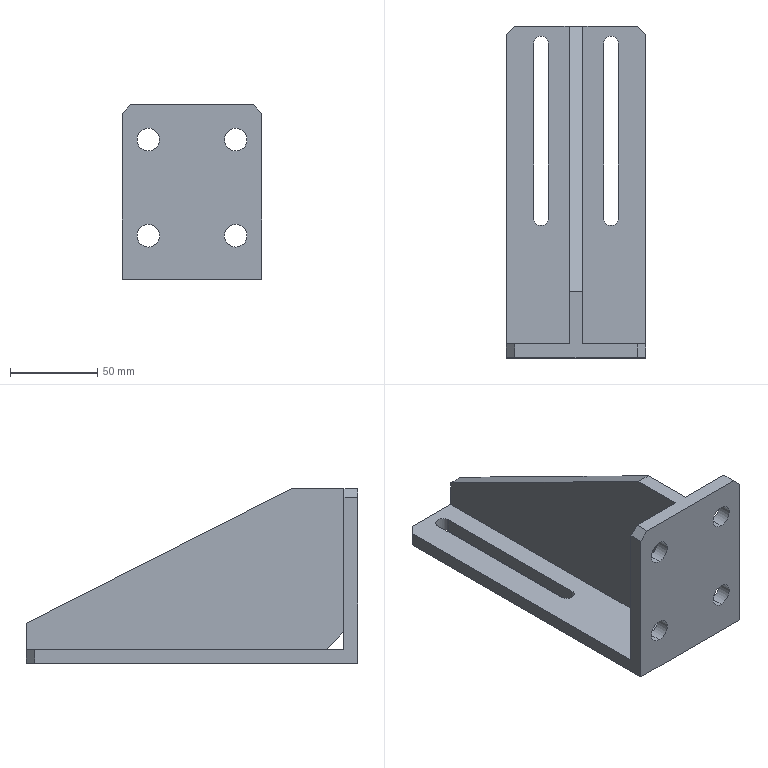Part | SolidWorks | features BaseBody 1 | 1 solid | 32 faces | box 80 x 190 x 100 mm | volume 248061 mm3 | plane 20 | cylinder 12 | commonest cylinder face diameters 13 x8 8.5 x4
STEP:
#1=CARTESIAN_POINT('',(-25.,-95.,18.5));
#2=VERTEX_POINT('',#1);
#3=CARTESIAN_POINT('',(-25.,-95.,31.5));
#4=VERTEX_POINT('',#3);
#5=CARTESIAN_POINT('',(-25.,-95.,25.));
#6=DIRECTION('',(0.,1.,0.));
#7=DIRECTION('',(0.,0.,1.));
#8=AXIS2_PLACEMENT_3D('',#5,#6,#7);
#9=CIRCLE('',#8,6.5);
#10=EDGE_CURVE('',#2,#4,#9,.T.);
#11=ORIENTED_EDGE('',*,*,#10,.F.);
#12=CARTESIAN_POINT('',(-25.,-87.,18.5));
#13=VERTEX_POINT('',#12);
#14=CARTESIAN_POINT('',(-25.,-87.,18.5));
#15=DIRECTION('',(0.,1.,0.));
#16=VECTOR('',#15,1000.);
#17=LINE('',#14,#16);
#18=EDGE_CURVE('',#2,#13,#17,.T.);
#19=ORIENTED_EDGE('',*,*,#18,.T.);
#20=CARTESIAN_POINT('',(-25.,-87.,31.5));
#21=VERTEX_POINT('',#20);
#22=CARTESIAN_POINT('',(-25.,-87.,25.));
#23=DIRECTION('',(0.,1.,0.));
#24=DIRECTION('',(0.,0.,1.));
#25=AXIS2_PLACEMENT_3D('',#22,#23,#24);
#26=CIRCLE('',#25,6.5);
#27=EDGE_CURVE('',#13,#21,#26,.T.);
#28=ORIENTED_EDGE('',*,*,#27,.T.);
#29=CARTESIAN_POINT('',(-25.,-87.,31.5));
#30=DIRECTION('',(0.,1.,0.));
#31=VECTOR('',#30,1000.);
#32=LINE('',#29,#31);
#33=EDGE_CURVE('',#4,#21,#32,.T.);
#34=ORIENTED_EDGE('',*,*,#33,.F.);
#35=EDGE_LOOP('',(#11,#19,#28,#34));
#36=FACE_OUTER_BOUND('',#35,.T.);
#37=CARTESIAN_POINT('',(-25.,-87.,25.));
#38=DIRECTION('',(0.,1.,0.));
#39=DIRECTION('',(0.,0.,1.));
#40=AXIS2_PLACEMENT_3D('',#37,#38,#39);
#41=CYLINDRICAL_SURFACE('',#40,6.5);
#42=ADVANCED_FACE('',(#36),#41,.F.);
#43=CARTESIAN_POINT('',(25.,-95.,18.5));
#44=VERTEX_POINT('',#43);
#45=CARTESIAN_POINT('',(25.,-95.,31.5));
#46=VERTEX_POINT('',#45);
#47=CARTESIAN_POINT('',(25.,-95.,25.));
#48=DIRECTION('',(0.,1.,0.));
#49=DIRECTION('',(0.,0.,1.));
#50=AXIS2_PLACEMENT_3D('',#47,#48,#49);
#51=CIRCLE('',#50,6.5);
#52=EDGE_CURVE('',#44,#46,#51,.T.);
#53=ORIENTED_EDGE('',*,*,#52,.F.);
#54=CARTESIAN_POINT('',(25.,-87.,18.5));
#55=VERTEX_POINT('',#54);
#56=CARTESIAN_POINT('',(25.,-87.,18.5));
#57=DIRECTION('',(0.,1.,0.));
#58=VECTOR('',#57,1000.);
#59=LINE('',#56,#58);
#60=EDGE_CURVE('',#44,#55,#59,.T.);
#61=ORIENTED_EDGE('',*,*,#60,.T.);
#62=CARTESIAN_POINT('',(25.,-87.,31.5));
#63=VERTEX_POINT('',#62);
#64=CARTESIAN_POINT('',(25.,-87.,25.));
#65=DIRECTION('',(0.,1.,0.));
#66=DIRECTION('',(0.,0.,1.));
#67=AXIS2_PLACEMENT_3D('',#64,#65,#66);
#68=CIRCLE('',#67,6.5);
#69=EDGE_CURVE('',#55,#63,#68,.T.);
#70=ORIENTED_EDGE('',*,*,#69,.T.);
#71=CARTESIAN_POINT('',(25.,-87.,31.5));
#72=DIRECTION('',(0.,1.,0.));
#73=VECTOR('',#72,1000.);
#74=LINE('',#71,#73);
#75=EDGE_CURVE('',#46,#63,#74,.T.);
#76=ORIENTED_EDGE('',*,*,#75,.F.);
#77=EDGE_LOOP('',(#53,#61,#70,#76));
#78=FACE_OUTER_BOUND('',#77,.T.);
#79=CARTESIAN_POINT('',(25.,-87.,25.));
#80=DIRECTION('',(0.,1.,0.));
#81=DIRECTION('',(0.,0.,1.));
#82=AXIS2_PLACEMENT_3D('',#79,#80,#81);
#83=CYLINDRICAL_SURFACE('',#82,6.5);
#84=ADVANCED_FACE('',(#78),#83,.F.);
#85=CARTESIAN_POINT('',(-25.,-95.,73.5));
#86=VERTEX_POINT('',#85);
#87=CARTESIAN_POINT('',(-25.,-95.,86.5));
#88=VERTEX_POINT('',#87);
#89=CARTESIAN_POINT('',(-25.,-95.,80.));
#90=DIRECTION('',(0.,1.,0.));
#91=DIRECTION('',(0.,0.,1.));
#92=AXIS2_PLACEMENT_3D('',#89,#90,#91);
#93=CIRCLE('',#92,6.5);
#94=EDGE_CURVE('',#86,#88,#93,.T.);
#95=ORIENTED_EDGE('',*,*,#94,.F.);
#96=CARTESIAN_POINT('',(-25.,-87.,73.5));
#97=VERTEX_POINT('',#96);
#98=CARTESIAN_POINT('',(-25.,-87.,73.5));
#99=DIRECTION('',(0.,1.,0.));
#100=VECTOR('',#99,1000.);
#101=LINE('',#98,#100);
#102=EDGE_CURVE('',#86,#97,#101,.T.);
#103=ORIENTED_EDGE('',*,*,#102,.T.);
#104=CARTESIAN_POINT('',(-25.,-87.,86.5));
#105=VERTEX_POINT('',#104);
#106=CARTESIAN_POINT('',(-25.,-87.,80.));
#107=DIRECTION('',(0.,1.,0.));
#108=DIRECTION('',(0.,0.,1.));
#109=AXIS2_PLACEMENT_3D('',#106,#107,#108);
#110=CIRCLE('',#109,6.5);
#111=EDGE_CURVE('',#97,#105,#110,.T.);
#112=ORIENTED_EDGE('',*,*,#111,.T.);
#113=CARTESIAN_POINT('',(-25.,-87.,86.5));
#114=DIRECTION('',(0.,1.,0.));
#115=VECTOR('',#114,1000.);
#116=LINE('',#113,#115);
#117=EDGE_CURVE('',#88,#105,#116,.T.);
#118=ORIENTED_EDGE('',*,*,#117,.F.);
#119=EDGE_LOOP('',(#95,#103,#112,#118));
#120=FACE_OUTER_BOUND('',#119,.T.);
#121=CARTESIAN_POINT('',(-25.,-87.,80.));
#122=DIRECTION('',(0.,1.,0.));
#123=DIRECTION('',(0.,0.,1.));
#124=AXIS2_PLACEMENT_3D('',#121,#122,#123);
#125=CYLINDRICAL_SURFACE('',#124,6.5);
#126=ADVANCED_FACE('',(#120),#125,.F.);
#127=CARTESIAN_POINT('',(25.,-95.,73.5));
#128=VERTEX_POINT('',#127);
#129=CARTESIAN_POINT('',(25.,-95.,86.5));
#130=VERTEX_POINT('',#129);
#131=CARTESIAN_POINT('',(25.,-95.,80.));
#132=DIRECTION('',(0.,1.,0.));
#133=DIRECTION('',(0.,0.,1.));
#134=AXIS2_PLACEMENT_3D('',#131,#132,#133);
#135=CIRCLE('',#134,6.5);
#136=EDGE_CURVE('',#128,#130,#135,.T.);
#137=ORIENTED_EDGE('',*,*,#136,.F.);
#138=CARTESIAN_POINT('',(25.,-87.,73.5));
#139=VERTEX_POINT('',#138);
#140=CARTESIAN_POINT('',(25.,-87.,73.5));
#141=DIRECTION('',(0.,1.,0.));
#142=VECTOR('',#141,1000.);
#143=LINE('',#140,#142);
#144=EDGE_CURVE('',#128,#139,#143,.T.);
#145=ORIENTED_EDGE('',*,*,#144,.T.);
#146=CARTESIAN_POINT('',(25.,-87.,86.5));
#147=VERTEX_POINT('',#146);
#148=CARTESIAN_POINT('',(25.,-87.,80.));
#149=DIRECTION('',(0.,1.,0.));
#150=DIRECTION('',(0.,0.,1.));
#151=AXIS2_PLACEMENT_3D('',#148,#149,#150);
#152=CIRCLE('',#151,6.5);
#153=EDGE_CURVE('',#139,#147,#152,.T.);
#154=ORIENTED_EDGE('',*,*,#153,.T.);
#155=CARTESIAN_POINT('',(25.,-87.,86.5));
#156=DIRECTION('',(0.,1.,0.));
#157=VECTOR('',#156,1000.);
#158=LINE('',#155,#157);
#159=EDGE_CURVE('',#130,#147,#158,.T.);
#160=ORIENTED_EDGE('',*,*,#159,.F.);
#161=EDGE_LOOP('',(#137,#145,#154,#160));
#162=FACE_OUTER_BOUND('',#161,.T.);
#163=CARTESIAN_POINT('',(25.,-87.,80.));
#164=DIRECTION('',(0.,1.,0.));
#165=DIRECTION('',(0.,0.,1.));
#166=AXIS2_PLACEMENT_3D('',#163,#164,#165);
#167=CYLINDRICAL_SURFACE('',#166,6.5);
#168=ADVANCED_FACE('',(#162),#167,.F.);
#169=CARTESIAN_POINT('',(-25.,-87.,25.));
#170=DIRECTION('',(0.,1.,0.));
#171=DIRECTION('',(0.,0.,1.));
#172=AXIS2_PLACEMENT_3D('',#169,#170,#171);
#173=CIRCLE('',#172,6.5);
#174=EDGE_CURVE('',#21,#13,#173,.T.);
#175=ORIENTED_EDGE('',*,*,#174,.F.);
#176=ORIENTED_EDGE('',*,*,#27,.F.);
#177=EDGE_LOOP('',(#175,#176));
#178=FACE_BOUND('',#177,.T.);
#179=CARTESIAN_POINT('',(25.,-87.,25.));
#180=DIRECTION('',(0.,1.,0.));
#181=DIRECTION('',(0.,0.,1.));
#182=AXIS2_PLACEMENT_3D('',#179,#180,#181);
#183=CIRCLE('',#182,6.5);
#184=EDGE_CURVE('',#63,#55,#183,.T.);
#185=ORIENTED_EDGE('',*,*,#184,.F.);
#186=ORIENTED_EDGE('',*,*,#69,.F.);
#187=EDGE_LOOP('',(#185,#186));
#188=FACE_BOUND('',#187,.T.);
#189=CARTESIAN_POINT('',(-40.,-87.,95.));
#190=VERTEX_POINT('',#189);
#191=CARTESIAN_POINT('',(-40.,-87.,8.));
#192=VERTEX_POINT('',#191);
#193=CARTESIAN_POINT('',(-40.,-87.,100.));
#194=DIRECTION('',(0.,0.,-1.));
#195=VECTOR('',#194,1000.);
#196=LINE('',#193,#195);
#197=EDGE_CURVE('',#190,#192,#196,.T.);
#198=ORIENTED_EDGE('',*,*,#197,.F.);
#199=CARTESIAN_POINT('',(-35.,-87.,100.));
#200=VERTEX_POINT('',#199);
#201=CARTESIAN_POINT('',(-35.,-87.,100.));
#202=DIRECTION('',(0.7071,0.,0.7071));
#203=VECTOR('',#202,1000.);
#204=LINE('',#201,#203);
#205=EDGE_CURVE('',#190,#200,#204,.T.);
#206=ORIENTED_EDGE('',*,*,#205,.T.);
#207=CARTESIAN_POINT('',(-4.,-87.,100.));
#208=VERTEX_POINT('',#207);
#209=CARTESIAN_POINT('',(-40.,-87.,100.));
#210=DIRECTION('',(-1.,0.,0.));
#211=VECTOR('',#210,1000.);
#212=LINE('',#209,#211);
#213=EDGE_CURVE('',#208,#200,#212,.T.);
#214=ORIENTED_EDGE('',*,*,#213,.F.);
#215=CARTESIAN_POINT('',(-4.,-87.,18.));
#216=VERTEX_POINT('',#215);
#217=CARTESIAN_POINT('',(-4.,-87.,18.));
#218=DIRECTION('',(0.,0.,1.));
#219=VECTOR('',#218,1000.);
#220=LINE('',#217,#219);
#221=EDGE_CURVE('',#216,#208,#220,.T.);
#222=ORIENTED_EDGE('',*,*,#221,.F.);
#223=CARTESIAN_POINT('',(4.,-87.,18.));
#224=VERTEX_POINT('',#223);
#225=CARTESIAN_POINT('',(-4.,-87.,18.));
#226=DIRECTION('',(1.,0.,0.));
#227=VECTOR('',#226,1000.);
#228=LINE('',#225,#227);
#229=EDGE_CURVE('',#216,#224,#228,.T.);
#230=ORIENTED_EDGE('',*,*,#229,.T.);
#231=CARTESIAN_POINT('',(4.,-87.,100.));
#232=VERTEX_POINT('',#231);
#233=CARTESIAN_POINT('',(4.,-87.,18.));
#234=DIRECTION('',(0.,0.,1.));
#235=VECTOR('',#234,1000.);
#236=LINE('',#233,#235);
#237=EDGE_CURVE('',#224,#232,#236,.T.);
#238=ORIENTED_EDGE('',*,*,#237,.T.);
#239=CARTESIAN_POINT('',(35.,-87.,100.));
#240=VERTEX_POINT('',#239);
#241=CARTESIAN_POINT('',(-40.,-87.,100.));
#242=DIRECTION('',(-1.,0.,0.));
#243=VECTOR('',#242,1000.);
#244=LINE('',#241,#243);
#245=EDGE_CURVE('',#240,#232,#244,.T.);
#246=ORIENTED_EDGE('',*,*,#245,.F.);
#247=CARTESIAN_POINT('',(40.,-87.,95.));
#248=VERTEX_POINT('',#247);
#249=CARTESIAN_POINT('',(35.,-87.,100.));
#250=DIRECTION('',(0.7071,0.,-0.7071));
#251=VECTOR('',#250,1000.);
#252=LINE('',#249,#251);
#253=EDGE_CURVE('',#240,#248,#252,.T.);
#254=ORIENTED_EDGE('',*,*,#253,.T.);
#255=CARTESIAN_POINT('',(40.,-87.,8.));
#256=VERTEX_POINT('',#255);
#257=CARTESIAN_POINT('',(40.,-87.,100.));
#258=DIRECTION('',(0.,0.,-1.));
#259=VECTOR('',#258,1000.);
#260=LINE('',#257,#259);
#261=EDGE_CURVE('',#248,#256,#260,.T.);
#262=ORIENTED_EDGE('',*,*,#261,.T.);
#263=CARTESIAN_POINT('',(-40.,-87.,8.));
#264=DIRECTION('',(-1.,0.,0.));
#265=VECTOR('',#264,1000.);
#266=LINE('',#263,#265);
#267=EDGE_CURVE('',#256,#192,#266,.T.);
#268=ORIENTED_EDGE('',*,*,#267,.T.);
#269=EDGE_LOOP('',(#198,#206,#214,#222,#230,#238,#246,#254,#262,#268));
#270=FACE_OUTER_BOUND('',#269,.T.);
#271=CARTESIAN_POINT('',(25.,-87.,80.));
#272=DIRECTION('',(0.,1.,0.));
#273=DIRECTION('',(0.,0.,1.));
#274=AXIS2_PLACEMENT_3D('',#271,#272,#273);
#275=CIRCLE('',#274,6.5);
#276=EDGE_CURVE('',#147,#139,#275,.T.);
#277=ORIENTED_EDGE('',*,*,#276,.F.);
#278=ORIENTED_EDGE('',*,*,#153,.F.);
#279=EDGE_LOOP('',(#277,#278));
#280=FACE_BOUND('',#279,.T.);
#281=CARTESIAN_POINT('',(-25.,-87.,80.));
#282=DIRECTION('',(0.,1.,0.));
#283=DIRECTION('',(0.,0.,1.));
#284=AXIS2_PLACEMENT_3D('',#281,#282,#283);
#285=CIRCLE('',#284,6.5);
#286=EDGE_CURVE('',#105,#97,#285,.T.);
#287=ORIENTED_EDGE('',*,*,#286,.F.);
#288=ORIENTED_EDGE('',*,*,#111,.F.);
#289=EDGE_LOOP('',(#287,#288));
#290=FACE_BOUND('',#289,.T.);
#291=CARTESIAN_POINT('',(-40.,-87.,100.));
#292=DIRECTION('',(0.,-1.,0.));
#293=DIRECTION('',(0.,0.,-1.));
#294=AXIS2_PLACEMENT_3D('',#291,#292,#293);
#295=PLANE('',#294);
#296=ADVANCED_FACE('',(#178,#188,#270,#280,#290),#295,.F.);
#297=CARTESIAN_POINT('',(15.75,85.,8.));
#298=VERTEX_POINT('',#297);
#299=CARTESIAN_POINT('',(15.75,-15.,8.));
#300=VERTEX_POINT('',#299);
#301=CARTESIAN_POINT('',(15.75,85.,8.));
#302=DIRECTION('',(0.,-1.,0.));
#303=VECTOR('',#302,1000.);
#304=LINE('',#301,#303);
#305=EDGE_CURVE('',#298,#300,#304,.T.);
#306=ORIENTED_EDGE('',*,*,#305,.F.);
#307=CARTESIAN_POINT('',(24.25,85.,8.));
#308=VERTEX_POINT('',#307);
#309=CARTESIAN_POINT('',(20.,85.,8.));
#310=DIRECTION('',(0.,0.,1.));
#311=DIRECTION('',(-1.,0.,0.));
#312=AXIS2_PLACEMENT_3D('',#309,#310,#311);
#313=CIRCLE('',#312,4.25);
#314=EDGE_CURVE('',#308,#298,#313,.T.);
#315=ORIENTED_EDGE('',*,*,#314,.F.);
#316=CARTESIAN_POINT('',(24.25,-15.,8.));
#317=VERTEX_POINT('',#316);
#318=CARTESIAN_POINT('',(24.25,85.,8.));
#319=DIRECTION('',(0.,1.,0.));
#320=VECTOR('',#319,1000.);
#321=LINE('',#318,#320);
#322=EDGE_CURVE('',#317,#308,#321,.T.);
#323=ORIENTED_EDGE('',*,*,#322,.F.);
#324=CARTESIAN_POINT('',(20.,-15.,8.));
#325=DIRECTION('',(0.,0.,1.));
#326=DIRECTION('',(-1.,0.,0.));
#327=AXIS2_PLACEMENT_3D('',#324,#325,#326);
#328=CIRCLE('',#327,4.25);
#329=EDGE_CURVE('',#300,#317,#328,.T.);
#330=ORIENTED_EDGE('',*,*,#329,.F.);
#331=EDGE_LOOP('',(#306,#315,#323,#330));
#332=FACE_BOUND('',#331,.T.);
#333=CARTESIAN_POINT('',(-24.25,85.,8.));
#334=VERTEX_POINT('',#333);
#335=CARTESIAN_POINT('',(-24.25,-15.,8.));
#336=VERTEX_POINT('',#335);
#337=CARTESIAN_POINT('',(-24.25,85.,8.));
#338=DIRECTION('',(0.,-1.,0.));
#339=VECTOR('',#338,1000.);
#340=LINE('',#337,#339);
#341=EDGE_CURVE('',#334,#336,#340,.T.);
#342=ORIENTED_EDGE('',*,*,#341,.F.);
#343=CARTESIAN_POINT('',(-15.75,85.,8.));
#344=VERTEX_POINT('',#343);
#345=CARTESIAN_POINT('',(-20.,85.,8.));
#346=DIRECTION('',(0.,0.,1.));
#347=DIRECTION('',(1.,0.,0.));
#348=AXIS2_PLACEMENT_3D('',#345,#346,#347);
#349=CIRCLE('',#348,4.25);
#350=EDGE_CURVE('',#344,#334,#349,.T.);
#351=ORIENTED_EDGE('',*,*,#350,.F.);
#352=CARTESIAN_POINT('',(-15.75,-15.,8.));
#353=VERTEX_POINT('',#352);
#354=CARTESIAN_POINT('',(-15.75,85.,8.));
#355=DIRECTION('',(0.,1.,0.));
#356=VECTOR('',#355,1000.);
#357=LINE('',#354,#356);
#358=EDGE_CURVE('',#353,#344,#357,.T.);
#359=ORIENTED_EDGE('',*,*,#358,.F.);
#360=CARTESIAN_POINT('',(-20.,-15.,8.));
#361=DIRECTION('',(0.,0.,1.));
#362=DIRECTION('',(1.,0.,0.));
#363=AXIS2_PLACEMENT_3D('',#360,#361,#362);
#364=CIRCLE('',#363,4.25);
#365=EDGE_CURVE('',#336,#353,#364,.T.);
#366=ORIENTED_EDGE('',*,*,#365,.F.);
#367=EDGE_LOOP('',(#342,#351,#359,#366));
#368=FACE_BOUND('',#367,.T.);
#369=CARTESIAN_POINT('',(40.,90.,8.));
#370=VERTEX_POINT('',#369);
#371=CARTESIAN_POINT('',(40.,95.,8.));
#372=DIRECTION('',(0.,1.,0.));
#373=VECTOR('',#372,1000.);
#374=LINE('',#371,#373);
#375=EDGE_CURVE('',#256,#370,#374,.T.);
#376=ORIENTED_EDGE('',*,*,#375,.T.);
#377=CARTESIAN_POINT('',(35.,95.,8.));
#378=VERTEX_POINT('',#377);
#379=CARTESIAN_POINT('',(35.,95.,8.));
#380=DIRECTION('',(-0.7071,0.7071,0.));
#381=VECTOR('',#380,1000.);
#382=LINE('',#379,#381);
#383=EDGE_CURVE('',#370,#378,#382,.T.);
#384=ORIENTED_EDGE('',*,*,#383,.T.);
#385=CARTESIAN_POINT('',(4.,95.,8.));
#386=VERTEX_POINT('',#385);
#387=CARTESIAN_POINT('',(40.,95.,8.));
#388=DIRECTION('',(-1.,0.,0.));
#389=VECTOR('',#388,1000.);
#390=LINE('',#387,#389);
#391=EDGE_CURVE('',#378,#386,#390,.T.);
#392=ORIENTED_EDGE('',*,*,#391,.T.);
#393=CARTESIAN_POINT('',(4.,-77.,8.));
#394=VERTEX_POINT('',#393);
#395=CARTESIAN_POINT('',(4.,95.,8.));
#396=DIRECTION('',(0.,-1.,0.));
#397=VECTOR('',#396,1000.);
#398=LINE('',#395,#397);
#399=EDGE_CURVE('',#386,#394,#398,.T.);
#400=ORIENTED_EDGE('',*,*,#399,.T.);
#401=CARTESIAN_POINT('',(-4.,-77.,8.));
#402=VERTEX_POINT('',#401);
#403=CARTESIAN_POINT('',(-4.,-77.,8.));
#404=DIRECTION('',(1.,0.,0.));
#405=VECTOR('',#404,1000.);
#406=LINE('',#403,#405);
#407=EDGE_CURVE('',#402,#394,#406,.T.);
#408=ORIENTED_EDGE('',*,*,#407,.F.);
#409=CARTESIAN_POINT('',(-4.,95.,8.));
#410=VERTEX_POINT('',#409);
#411=CARTESIAN_POINT('',(-4.,95.,8.));
#412=DIRECTION('',(0.,-1.,0.));
#413=VECTOR('',#412,1000.);
#414=LINE('',#411,#413);
#415=EDGE_CURVE('',#410,#402,#414,.T.);
#416=ORIENTED_EDGE('',*,*,#415,.F.);
#417=CARTESIAN_POINT('',(-35.,95.,8.));
#418=VERTEX_POINT('',#417);
#419=CARTESIAN_POINT('',(40.,95.,8.));
#420=DIRECTION('',(-1.,0.,0.));
#421=VECTOR('',#420,1000.);
#422=LINE('',#419,#421);
#423=EDGE_CURVE('',#410,#418,#422,.T.);
#424=ORIENTED_EDGE('',*,*,#423,.T.);
#425=CARTESIAN_POINT('',(-40.,90.,8.));
#426=VERTEX_POINT('',#425);
#427=CARTESIAN_POINT('',(-40.,90.,8.));
#428=DIRECTION('',(-0.7071,-0.7071,0.));
#429=VECTOR('',#428,1000.);
#430=LINE('',#427,#429);
#431=EDGE_CURVE('',#418,#426,#430,.T.);
#432=ORIENTED_EDGE('',*,*,#431,.T.);
#433=CARTESIAN_POINT('',(-40.,95.,8.));
#434=DIRECTION('',(0.,-1.,0.));
#435=VECTOR('',#434,1000.);
#436=LINE('',#433,#435);
#437=EDGE_CURVE('',#426,#192,#436,.T.);
#438=ORIENTED_EDGE('',*,*,#437,.T.);
#439=ORIENTED_EDGE('',*,*,#267,.F.);
#440=EDGE_LOOP('',(#376,#384,#392,#400,#408,#416,#424,#432,#438,#439));
#441=FACE_OUTER_BOUND('',#440,.T.);
#442=CARTESIAN_POINT('',(0.,0.,8.));
#443=DIRECTION('',(0.,0.,-1.));
#444=DIRECTION('',(-1.,0.,0.));
#445=AXIS2_PLACEMENT_3D('',#442,#443,#444);
#446=PLANE('',#445);
#447=ADVANCED_FACE('',(#332,#368,#441),#446,.F.);
#448=CARTESIAN_POINT('',(-40.,-95.,95.));
#449=VERTEX_POINT('',#448);
#450=CARTESIAN_POINT('',(-40.,-95.,0.));
#451=VERTEX_POINT('',#450);
#452=CARTESIAN_POINT('',(-40.,-95.,8.));
#453=DIRECTION('',(0.,0.,-1.));
#454=VECTOR('',#453,1000.);
#455=LINE('',#452,#454);
#456=EDGE_CURVE('',#449,#451,#455,.T.);
#457=ORIENTED_EDGE('',*,*,#456,.F.);
#458=CARTESIAN_POINT('',(-40.,95.,95.));
#459=DIRECTION('',(0.,1.,0.));
#460=VECTOR('',#459,1000.);
#461=LINE('',#458,#460);
#462=EDGE_CURVE('',#449,#190,#461,.T.);
#463=ORIENTED_EDGE('',*,*,#462,.T.);
#464=ORIENTED_EDGE('',*,*,#197,.T.);
#465=ORIENTED_EDGE('',*,*,#437,.F.);
#466=CARTESIAN_POINT('',(-40.,90.,0.));
#467=VERTEX_POINT('',#466);
#468=CARTESIAN_POINT('',(-40.,90.,8.));
#469=DIRECTION('',(0.,0.,-1.));
#470=VECTOR('',#469,1000.);
#471=LINE('',#468,#470);
#472=EDGE_CURVE('',#426,#467,#471,.T.);
#473=ORIENTED_EDGE('',*,*,#472,.T.);
#474=CARTESIAN_POINT('',(-40.,95.,0.));
#475=DIRECTION('',(0.,-1.,0.));
#476=VECTOR('',#475,1000.);
#477=LINE('',#474,#476);
#478=EDGE_CURVE('',#467,#451,#477,.T.);
#479=ORIENTED_EDGE('',*,*,#478,.T.);
#480=EDGE_LOOP('',(#457,#463,#464,#465,#473,#479));
#481=FACE_OUTER_BOUND('',#480,.T.);
#482=CARTESIAN_POINT('',(-40.,95.,8.));
#483=DIRECTION('',(1.,0.,0.));
#484=DIRECTION('',(0.,1.,0.));
#485=AXIS2_PLACEMENT_3D('',#482,#483,#484);
#486=PLANE('',#485);
#487=ADVANCED_FACE('',(#481),#486,.F.);
#488=CARTESIAN_POINT('',(-25.,-95.,25.));
#489=DIRECTION('',(0.,1.,0.));
#490=DIRECTION('',(0.,0.,1.));
#491=AXIS2_PLACEMENT_3D('',#488,#489,#490);
#492=CIRCLE('',#491,6.5);
#493=EDGE_CURVE('',#4,#2,#492,.T.);
#494=ORIENTED_EDGE('',*,*,#493,.T.);
#495=ORIENTED_EDGE('',*,*,#10,.T.);
#496=EDGE_LOOP('',(#494,#495));
#497=FACE_BOUND('',#496,.T.);
#498=CARTESIAN_POINT('',(25.,-95.,25.));
#499=DIRECTION('',(0.,1.,0.));
#500=DIRECTION('',(0.,0.,1.));
#501=AXIS2_PLACEMENT_3D('',#498,#499,#500);
#502=CIRCLE('',#501,6.5);
#503=EDGE_CURVE('',#46,#44,#502,.T.);
#504=ORIENTED_EDGE('',*,*,#503,.T.);
#505=ORIENTED_EDGE('',*,*,#52,.T.);
#506=EDGE_LOOP('',(#504,#505));
#507=FACE_BOUND('',#506,.T.);
#508=CARTESIAN_POINT('',(-25.,-95.,80.));
#509=DIRECTION('',(0.,1.,0.));
#510=DIRECTION('',(0.,0.,1.));
#511=AXIS2_PLACEMENT_3D('',#508,#509,#510);
#512=CIRCLE('',#511,6.5);
#513=EDGE_CURVE('',#88,#86,#512,.T.);
#514=ORIENTED_EDGE('',*,*,#513,.T.);
#515=ORIENTED_EDGE('',*,*,#94,.T.);
#516=EDGE_LOOP('',(#514,#515));
#517=FACE_BOUND('',#516,.T.);
#518=CARTESIAN_POINT('',(25.,-95.,80.));
#519=DIRECTION('',(0.,1.,0.));
#520=DIRECTION('',(0.,0.,1.));
#521=AXIS2_PLACEMENT_3D('',#518,#519,#520);
#522=CIRCLE('',#521,6.5);
#523=EDGE_CURVE('',#130,#128,#522,.T.);
#524=ORIENTED_EDGE('',*,*,#523,.T.);
#525=ORIENTED_EDGE('',*,*,#136,.T.);
#526=EDGE_LOOP('',(#524,#525));
#527=FACE_BOUND('',#526,.T.);
#528=CARTESIAN_POINT('',(-35.,-95.,100.));
#529=VERTEX_POINT('',#528);
#530=CARTESIAN_POINT('',(35.,-95.,100.));
#531=VERTEX_POINT('',#530);
#532=CARTESIAN_POINT('',(-40.,-95.,100.));
#533=DIRECTION('',(1.,0.,0.));
#534=VECTOR('',#533,1000.);
#535=LINE('',#532,#534);
#536=EDGE_CURVE('',#529,#531,#535,.T.);
#537=ORIENTED_EDGE('',*,*,#536,.F.);
#538=CARTESIAN_POINT('',(-35.,-95.,100.));
#539=DIRECTION('',(-0.7071,0.,-0.7071));
#540=VECTOR('',#539,1000.);
#541=LINE('',#538,#540);
#542=EDGE_CURVE('',#529,#449,#541,.T.);
#543=ORIENTED_EDGE('',*,*,#542,.T.);
#544=ORIENTED_EDGE('',*,*,#456,.T.);
#545=CARTESIAN_POINT('',(40.,-95.,0.));
#546=VERTEX_POINT('',#545);
#547=CARTESIAN_POINT('',(40.,-95.,0.));
#548=DIRECTION('',(1.,0.,0.));
#549=VECTOR('',#548,1000.);
#550=LINE('',#547,#549);
#551=EDGE_CURVE('',#451,#546,#550,.T.);
#552=ORIENTED_EDGE('',*,*,#551,.T.);
#553=CARTESIAN_POINT('',(40.,-95.,95.));
#554=VERTEX_POINT('',#553);
#555=CARTESIAN_POINT('',(40.,-95.,8.));
#556=DIRECTION('',(0.,0.,-1.));
#557=VECTOR('',#556,1000.);
#558=LINE('',#555,#557);
#559=EDGE_CURVE('',#554,#546,#558,.T.);
#560=ORIENTED_EDGE('',*,*,#559,.F.);
#561=CARTESIAN_POINT('',(35.,-95.,100.));
#562=DIRECTION('',(-0.7071,0.,0.7071));
#563=VECTOR('',#562,1000.);
#564=LINE('',#561,#563);
#565=EDGE_CURVE('',#554,#531,#564,.T.);
#566=ORIENTED_EDGE('',*,*,#565,.T.);
#567=EDGE_LOOP('',(#537,#543,#544,#552,#560,#566));
#568=FACE_OUTER_BOUND('',#567,.T.);
#569=CARTESIAN_POINT('',(40.,-95.,8.));
#570=DIRECTION('',(0.,1.,0.));
#571=DIRECTION('',(0.,0.,1.));
#572=AXIS2_PLACEMENT_3D('',#569,#570,#571);
#573=PLANE('',#572);
#574=ADVANCED_FACE('',(#497,#507,#517,#527,#568),#573,.F.);
#575=ORIENTED_EDGE('',*,*,#261,.F.);
#576=CARTESIAN_POINT('',(40.,95.,95.));
#577=DIRECTION('',(0.,-1.,0.));
#578=VECTOR('',#577,1000.);
#579=LINE('',#576,#578);
#580=EDGE_CURVE('',#248,#554,#579,.T.);
#581=ORIENTED_EDGE('',*,*,#580,.T.);
#582=ORIENTED_EDGE('',*,*,#559,.T.);
#583=CARTESIAN_POINT('',(40.,90.,0.));
#584=VERTEX_POINT('',#583);
#585=CARTESIAN_POINT('',(40.,95.,0.));
#586=DIRECTION('',(0.,1.,0.));
#587=VECTOR('',#586,1000.);
#588=LINE('',#585,#587);
#589=EDGE_CURVE('',#546,#584,#588,.T.);
#590=ORIENTED_EDGE('',*,*,#589,.T.);
#591=CARTESIAN_POINT('',(40.,90.,8.));
#592=DIRECTION('',(0.,0.,1.));
#593=VECTOR('',#592,1000.);
#594=LINE('',#591,#593);
#595=EDGE_CURVE('',#584,#370,#594,.T.);
#596=ORIENTED_EDGE('',*,*,#595,.T.);
#597=ORIENTED_EDGE('',*,*,#375,.F.);
#598=EDGE_LOOP('',(#575,#581,#582,#590,#596,#597));
#599=FACE_OUTER_BOUND('',#598,.T.);
#600=CARTESIAN_POINT('',(40.,95.,8.));
#601=DIRECTION('',(-1.,0.,0.));
#602=DIRECTION('',(0.,-1.,0.));
#603=AXIS2_PLACEMENT_3D('',#600,#601,#602);
#604=PLANE('',#603);
#605=ADVANCED_FACE('',(#599),#604,.F.);
#606=ORIENTED_EDGE('',*,*,#391,.F.);
#607=CARTESIAN_POINT('',(35.,95.,0.));
#608=VERTEX_POINT('',#607);
#609=CARTESIAN_POINT('',(35.,95.,8.));
#610=DIRECTION('',(0.,0.,-1.));
#611=VECTOR('',#610,1000.);
#612=LINE('',#609,#611);
#613=EDGE_CURVE('',#378,#608,#612,.T.);
#614=ORIENTED_EDGE('',*,*,#613,.T.);
#615=CARTESIAN_POINT('',(-35.,95.,0.));
#616=VERTEX_POINT('',#615);
#617=CARTESIAN_POINT('',(40.,95.,0.));
#618=DIRECTION('',(-1.,0.,0.));
#619=VECTOR('',#618,1000.);
#620=LINE('',#617,#619);
#621=EDGE_CURVE('',#608,#616,#620,.T.);
#622=ORIENTED_EDGE('',*,*,#621,.T.);
#623=CARTESIAN_POINT('',(-35.,95.,8.));
#624=DIRECTION('',(0.,0.,1.));
#625=VECTOR('',#624,1000.);
#626=LINE('',#623,#625);
#627=EDGE_CURVE('',#616,#418,#626,.T.);
#628=ORIENTED_EDGE('',*,*,#627,.T.);
#629=ORIENTED_EDGE('',*,*,#423,.F.);
#630=CARTESIAN_POINT('',(-4.,95.,23.));
#631=VERTEX_POINT('',#630);
#632=CARTESIAN_POINT('',(-4.,95.,8.));
#633=DIRECTION('',(0.,0.,-1.));
#634=VECTOR('',#633,1000.);
#635=LINE('',#632,#634);
#636=EDGE_CURVE('',#631,#410,#635,.T.);
#637=ORIENTED_EDGE('',*,*,#636,.F.);
#638=CARTESIAN_POINT('',(4.,95.,23.));
#639=VERTEX_POINT('',#638);
#640=CARTESIAN_POINT('',(-4.,95.,23.));
#641=DIRECTION('',(1.,0.,0.));
#642=VECTOR('',#641,1000.);
#643=LINE('',#640,#642);
#644=EDGE_CURVE('',#631,#639,#643,.T.);
#645=ORIENTED_EDGE('',*,*,#644,.T.);
#646=CARTESIAN_POINT('',(4.,95.,8.));
#647=DIRECTION('',(0.,0.,-1.));
#648=VECTOR('',#647,1000.);
#649=LINE('',#646,#648);
#650=EDGE_CURVE('',#639,#386,#649,.T.);
#651=ORIENTED_EDGE('',*,*,#650,.T.);
#652=EDGE_LOOP('',(#606,#614,#622,#628,#629,#637,#645,#651));
#653=FACE_OUTER_BOUND('',#652,.T.);
#654=CARTESIAN_POINT('',(40.,95.,8.));
#655=DIRECTION('',(0.,-1.,0.));
#656=DIRECTION('',(0.,0.,-1.));
#657=AXIS2_PLACEMENT_3D('',#654,#655,#656);
#658=PLANE('',#657);
#659=ADVANCED_FACE('',(#653),#658,.F.);
#660=CARTESIAN_POINT('',(24.25,85.,0.));
#661=VERTEX_POINT('',#660);
#662=CARTESIAN_POINT('',(15.75,85.,0.));
#663=VERTEX_POINT('',#662);
#664=CARTESIAN_POINT('',(20.,85.,0.));
#665=DIRECTION('',(0.,0.,1.));
#666=DIRECTION('',(-1.,0.,0.));
#667=AXIS2_PLACEMENT_3D('',#664,#665,#666);
#668=CIRCLE('',#667,4.25);
#669=EDGE_CURVE('',#661,#663,#668,.T.);
#670=ORIENTED_EDGE('',*,*,#669,.T.);
#671=CARTESIAN_POINT('',(15.75,-15.,0.));
#672=VERTEX_POINT('',#671);
#673=CARTESIAN_POINT('',(15.75,85.,0.));
#674=DIRECTION('',(0.,-1.,0.));
#675=VECTOR('',#674,1000.);
#676=LINE('',#673,#675);
#677=EDGE_CURVE('',#663,#672,#676,.T.);
#678=ORIENTED_EDGE('',*,*,#677,.T.);
#679=CARTESIAN_POINT('',(24.25,-15.,0.));
#680=VERTEX_POINT('',#679);
#681=CARTESIAN_POINT('',(20.,-15.,0.));
#682=DIRECTION('',(0.,0.,1.));
#683=DIRECTION('',(-1.,0.,0.));
#684=AXIS2_PLACEMENT_3D('',#681,#682,#683);
#685=CIRCLE('',#684,4.25);
#686=EDGE_CURVE('',#672,#680,#685,.T.);
#687=ORIENTED_EDGE('',*,*,#686,.T.);
#688=CARTESIAN_POINT('',(24.25,85.,0.));
#689=DIRECTION('',(0.,1.,0.));
#690=VECTOR('',#689,1000.);
#691=LINE('',#688,#690);
#692=EDGE_CURVE('',#680,#661,#691,.T.);
#693=ORIENTED_EDGE('',*,*,#692,.T.);
#694=EDGE_LOOP('',(#670,#678,#687,#693));
#695=FACE_BOUND('',#694,.T.);
#696=CARTESIAN_POINT('',(-15.75,85.,0.));
#697=VERTEX_POINT('',#696);
#698=CARTESIAN_POINT('',(-24.25,85.,0.));
#699=VERTEX_POINT('',#698);
#700=CARTESIAN_POINT('',(-20.,85.,0.));
#701=DIRECTION('',(0.,0.,1.));
#702=DIRECTION('',(1.,0.,0.));
#703=AXIS2_PLACEMENT_3D('',#700,#701,#702);
#704=CIRCLE('',#703,4.25);
#705=EDGE_CURVE('',#697,#699,#704,.T.);
#706=ORIENTED_EDGE('',*,*,#705,.T.);
#707=CARTESIAN_POINT('',(-24.25,-15.,0.));
#708=VERTEX_POINT('',#707);
#709=CARTESIAN_POINT('',(-24.25,85.,0.));
#710=DIRECTION('',(0.,-1.,0.));
#711=VECTOR('',#710,1000.);
#712=LINE('',#709,#711);
#713=EDGE_CURVE('',#699,#708,#712,.T.);
#714=ORIENTED_EDGE('',*,*,#713,.T.);
#715=CARTESIAN_POINT('',(-15.75,-15.,0.));
#716=VERTEX_POINT('',#715);
#717=CARTESIAN_POINT('',(-20.,-15.,0.));
#718=DIRECTION('',(0.,0.,1.));
#719=DIRECTION('',(1.,0.,0.));
#720=AXIS2_PLACEMENT_3D('',#717,#718,#719);
#721=CIRCLE('',#720,4.25);
#722=EDGE_CURVE('',#708,#716,#721,.T.);
#723=ORIENTED_EDGE('',*,*,#722,.T.);
#724=CARTESIAN_POINT('',(-15.75,85.,0.));
#725=DIRECTION('',(0.,1.,0.));
#726=VECTOR('',#725,1000.);
#727=LINE('',#724,#726);
#728=EDGE_CURVE('',#716,#697,#727,.T.);
#729=ORIENTED_EDGE('',*,*,#728,.T.);
#730=EDGE_LOOP('',(#706,#714,#723,#729));
#731=FACE_BOUND('',#730,.T.);
#732=ORIENTED_EDGE('',*,*,#621,.F.);
#733=CARTESIAN_POINT('',(65.,65.,0.));
#734=DIRECTION('',(0.7071,-0.7071,0.));
#735=VECTOR('',#734,1000.);
#736=LINE('',#733,#735);
#737=EDGE_CURVE('',#608,#584,#736,.T.);
#738=ORIENTED_EDGE('',*,*,#737,.T.);
#739=ORIENTED_EDGE('',*,*,#589,.F.);
#740=ORIENTED_EDGE('',*,*,#551,.F.);
#741=ORIENTED_EDGE('',*,*,#478,.F.);
#742=CARTESIAN_POINT('',(-65.,65.,0.));
#743=DIRECTION('',(0.7071,0.7071,0.));
#744=VECTOR('',#743,1000.);
#745=LINE('',#742,#744);
#746=EDGE_CURVE('',#467,#616,#745,.T.);
#747=ORIENTED_EDGE('',*,*,#746,.T.);
#748=EDGE_LOOP('',(#732,#738,#739,#740,#741,#747));
#749=FACE_OUTER_BOUND('',#748,.T.);
#750=CARTESIAN_POINT('',(0.,0.,0.));
#751=DIRECTION('',(0.,0.,-1.));
#752=DIRECTION('',(-1.,0.,0.));
#753=AXIS2_PLACEMENT_3D('',#750,#751,#752);
#754=PLANE('',#753);
#755=ADVANCED_FACE('',(#695,#731,#749),#754,.T.);
#756=ORIENTED_EDGE('',*,*,#213,.T.);
#757=CARTESIAN_POINT('',(-35.,0.,100.));
#758=DIRECTION('',(0.,-1.,0.));
#759=VECTOR('',#758,1000.);
#760=LINE('',#757,#759);
#761=EDGE_CURVE('',#200,#529,#760,.T.);
#762=ORIENTED_EDGE('',*,*,#761,.T.);
#763=ORIENTED_EDGE('',*,*,#536,.T.);
#764=CARTESIAN_POINT('',(35.,0.,100.));
#765=DIRECTION('',(0.,1.,0.));
#766=VECTOR('',#765,1000.);
#767=LINE('',#764,#766);
#768=EDGE_CURVE('',#531,#240,#767,.T.);
#769=ORIENTED_EDGE('',*,*,#768,.T.);
#770=ORIENTED_EDGE('',*,*,#245,.T.);
#771=CARTESIAN_POINT('',(4.,-57.,100.));
#772=VERTEX_POINT('',#771);
#773=CARTESIAN_POINT('',(4.,-57.,100.));
#774=DIRECTION('',(0.,1.,0.));
#775=VECTOR('',#774,1000.);
#776=LINE('',#773,#775);
#777=EDGE_CURVE('',#232,#772,#776,.T.);
#778=ORIENTED_EDGE('',*,*,#777,.T.);
#779=CARTESIAN_POINT('',(-4.,-57.,100.));
#780=VERTEX_POINT('',#779);
#781=CARTESIAN_POINT('',(-4.,-57.,100.));
#782=DIRECTION('',(1.,0.,0.));
#783=VECTOR('',#782,1000.);
#784=LINE('',#781,#783);
#785=EDGE_CURVE('',#780,#772,#784,.T.);
#786=ORIENTED_EDGE('',*,*,#785,.F.);
#787=CARTESIAN_POINT('',(-4.,-57.,100.));
#788=DIRECTION('',(0.,1.,0.));
#789=VECTOR('',#788,1000.);
#790=LINE('',#787,#789);
#791=EDGE_CURVE('',#208,#780,#790,.T.);
#792=ORIENTED_EDGE('',*,*,#791,.F.);
#793=EDGE_LOOP('',(#756,#762,#763,#769,#770,#778,#786,#792));
#794=FACE_OUTER_BOUND('',#793,.T.);
#795=CARTESIAN_POINT('',(0.,0.,100.));
#796=DIRECTION('',(0.,0.,-1.));
#797=DIRECTION('',(-1.,0.,0.));
#798=AXIS2_PLACEMENT_3D('',#795,#796,#797);
#799=PLANE('',#798);
#800=ADVANCED_FACE('',(#794),#799,.F.);
#801=CARTESIAN_POINT('',(4.,-77.,8.));
#802=DIRECTION('',(0.,-0.7071,0.7071));
#803=VECTOR('',#802,1000.);
#804=LINE('',#801,#803);
#805=EDGE_CURVE('',#394,#224,#804,.T.);
#806=ORIENTED_EDGE('',*,*,#805,.T.);
#807=ORIENTED_EDGE('',*,*,#229,.F.);
#808=CARTESIAN_POINT('',(-4.,-77.,8.));
#809=DIRECTION('',(0.,-0.7071,0.7071));
#810=VECTOR('',#809,1000.);
#811=LINE('',#808,#810);
#812=EDGE_CURVE('',#402,#216,#811,.T.);
#813=ORIENTED_EDGE('',*,*,#812,.F.);
#814=ORIENTED_EDGE('',*,*,#407,.T.);
#815=EDGE_LOOP('',(#806,#807,#813,#814));
#816=FACE_OUTER_BOUND('',#815,.T.);
#817=CARTESIAN_POINT('',(-4.,-77.,8.));
#818=DIRECTION('',(0.,0.7071,0.7071));
#819=DIRECTION('',(0.,-0.7071,0.7071));
#820=AXIS2_PLACEMENT_3D('',#817,#818,#819);
#821=PLANE('',#820);
#822=ADVANCED_FACE('',(#816),#821,.F.);
#823=CARTESIAN_POINT('',(4.,95.,23.));
#824=DIRECTION('',(0.,0.8921,-0.4519));
#825=VECTOR('',#824,1000.);
#826=LINE('',#823,#825);
#827=EDGE_CURVE('',#772,#639,#826,.T.);
#828=ORIENTED_EDGE('',*,*,#827,.T.);
#829=ORIENTED_EDGE('',*,*,#644,.F.);
#830=CARTESIAN_POINT('',(-4.,95.,23.));
#831=DIRECTION('',(0.,0.8921,-0.4519));
#832=VECTOR('',#831,1000.);
#833=LINE('',#830,#832);
#834=EDGE_CURVE('',#780,#631,#833,.T.);
#835=ORIENTED_EDGE('',*,*,#834,.F.);
#836=ORIENTED_EDGE('',*,*,#785,.T.);
#837=EDGE_LOOP('',(#828,#829,#835,#836));
#838=FACE_OUTER_BOUND('',#837,.T.);
#839=CARTESIAN_POINT('',(-4.,95.,23.));
#840=DIRECTION('',(0.,-0.4519,-0.8921));
#841=DIRECTION('',(0.,0.8921,-0.4519));
#842=AXIS2_PLACEMENT_3D('',#839,#840,#841);
#843=PLANE('',#842);
#844=ADVANCED_FACE('',(#838),#843,.F.);
#845=ORIENTED_EDGE('',*,*,#415,.T.);
#846=ORIENTED_EDGE('',*,*,#812,.T.);
#847=ORIENTED_EDGE('',*,*,#221,.T.);
#848=ORIENTED_EDGE('',*,*,#791,.T.);
#849=ORIENTED_EDGE('',*,*,#834,.T.);
#850=ORIENTED_EDGE('',*,*,#636,.T.);
#851=EDGE_LOOP('',(#845,#846,#847,#848,#849,#850));
#852=FACE_OUTER_BOUND('',#851,.T.);
#853=CARTESIAN_POINT('',(-4.,0.,0.));
#854=DIRECTION('',(-1.,0.,0.));
#855=DIRECTION('',(0.,-1.,0.));
#856=AXIS2_PLACEMENT_3D('',#853,#854,#855);
#857=PLANE('',#856);
#858=ADVANCED_FACE('',(#852),#857,.T.);
#859=ORIENTED_EDGE('',*,*,#399,.F.);
#860=ORIENTED_EDGE('',*,*,#650,.F.);
#861=ORIENTED_EDGE('',*,*,#827,.F.);
#862=ORIENTED_EDGE('',*,*,#777,.F.);
#863=ORIENTED_EDGE('',*,*,#237,.F.);
#864=ORIENTED_EDGE('',*,*,#805,.F.);
#865=EDGE_LOOP('',(#859,#860,#861,#862,#863,#864));
#866=FACE_OUTER_BOUND('',#865,.T.);
#867=CARTESIAN_POINT('',(4.,0.,0.));
#868=DIRECTION('',(-1.,0.,0.));
#869=DIRECTION('',(0.,-1.,0.));
#870=AXIS2_PLACEMENT_3D('',#867,#868,#869);
#871=PLANE('',#870);
#872=ADVANCED_FACE('',(#866),#871,.F.);
#873=ORIENTED_EDGE('',*,*,#205,.F.);
#874=ORIENTED_EDGE('',*,*,#462,.F.);
#875=ORIENTED_EDGE('',*,*,#542,.F.);
#876=ORIENTED_EDGE('',*,*,#761,.F.);
#877=EDGE_LOOP('',(#873,#874,#875,#876));
#878=FACE_OUTER_BOUND('',#877,.T.);
#879=CARTESIAN_POINT('',(-35.,0.,100.));
#880=DIRECTION('',(0.7071,0.,-0.7071));
#881=DIRECTION('',(0.,-1.,0.));
#882=AXIS2_PLACEMENT_3D('',#879,#880,#881);
#883=PLANE('',#882);
#884=ADVANCED_FACE('',(#878),#883,.F.);
#885=ORIENTED_EDGE('',*,*,#565,.F.);
#886=ORIENTED_EDGE('',*,*,#580,.F.);
#887=ORIENTED_EDGE('',*,*,#253,.F.);
#888=ORIENTED_EDGE('',*,*,#768,.F.);
#889=EDGE_LOOP('',(#885,#886,#887,#888));
#890=FACE_OUTER_BOUND('',#889,.T.);
#891=CARTESIAN_POINT('',(35.,0.,100.));
#892=DIRECTION('',(-0.7071,0.,-0.7071));
#893=DIRECTION('',(0.,1.,0.));
#894=AXIS2_PLACEMENT_3D('',#891,#892,#893);
#895=PLANE('',#894);
#896=ADVANCED_FACE('',(#890),#895,.F.);
#897=ORIENTED_EDGE('',*,*,#383,.F.);
#898=ORIENTED_EDGE('',*,*,#595,.F.);
#899=ORIENTED_EDGE('',*,*,#737,.F.);
#900=ORIENTED_EDGE('',*,*,#613,.F.);
#901=EDGE_LOOP('',(#897,#898,#899,#900));
#902=FACE_OUTER_BOUND('',#901,.T.);
#903=CARTESIAN_POINT('',(35.,95.,8.));
#904=DIRECTION('',(-0.7071,-0.7071,0.));
#905=DIRECTION('',(0.,0.,-1.));
#906=AXIS2_PLACEMENT_3D('',#903,#904,#905);
#907=PLANE('',#906);
#908=ADVANCED_FACE('',(#902),#907,.F.);
#909=ORIENTED_EDGE('',*,*,#431,.F.);
#910=ORIENTED_EDGE('',*,*,#627,.F.);
#911=ORIENTED_EDGE('',*,*,#746,.F.);
#912=ORIENTED_EDGE('',*,*,#472,.F.);
#913=EDGE_LOOP('',(#909,#910,#911,#912));
#914=FACE_OUTER_BOUND('',#913,.T.);
#915=CARTESIAN_POINT('',(-40.,90.,8.));
#916=DIRECTION('',(0.7071,-0.7071,0.));
#917=DIRECTION('',(0.,0.,-1.));
#918=AXIS2_PLACEMENT_3D('',#915,#916,#917);
#919=PLANE('',#918);
#920=ADVANCED_FACE('',(#914),#919,.F.);
#921=ORIENTED_EDGE('',*,*,#144,.F.);
#922=ORIENTED_EDGE('',*,*,#523,.F.);
#923=ORIENTED_EDGE('',*,*,#159,.T.);
#924=ORIENTED_EDGE('',*,*,#276,.T.);
#925=EDGE_LOOP('',(#921,#922,#923,#924));
#926=FACE_OUTER_BOUND('',#925,.T.);
#927=CARTESIAN_POINT('',(25.,-87.,80.));
#928=DIRECTION('',(0.,1.,0.));
#929=DIRECTION('',(0.,0.,1.));
#930=AXIS2_PLACEMENT_3D('',#927,#928,#929);
#931=CYLINDRICAL_SURFACE('',#930,6.5);
#932=ADVANCED_FACE('',(#926),#931,.F.);
#933=ORIENTED_EDGE('',*,*,#102,.F.);
#934=ORIENTED_EDGE('',*,*,#513,.F.);
#935=ORIENTED_EDGE('',*,*,#117,.T.);
#936=ORIENTED_EDGE('',*,*,#286,.T.);
#937=EDGE_LOOP('',(#933,#934,#935,#936));
#938=FACE_OUTER_BOUND('',#937,.T.);
#939=CARTESIAN_POINT('',(-25.,-87.,80.));
#940=DIRECTION('',(0.,1.,0.));
#941=DIRECTION('',(0.,0.,1.));
#942=AXIS2_PLACEMENT_3D('',#939,#940,#941);
#943=CYLINDRICAL_SURFACE('',#942,6.5);
#944=ADVANCED_FACE('',(#938),#943,.F.);
#945=ORIENTED_EDGE('',*,*,#60,.F.);
#946=ORIENTED_EDGE('',*,*,#503,.F.);
#947=ORIENTED_EDGE('',*,*,#75,.T.);
#948=ORIENTED_EDGE('',*,*,#184,.T.);
#949=EDGE_LOOP('',(#945,#946,#947,#948));
#950=FACE_OUTER_BOUND('',#949,.T.);
#951=CARTESIAN_POINT('',(25.,-87.,25.));
#952=DIRECTION('',(0.,1.,0.));
#953=DIRECTION('',(0.,0.,1.));
#954=AXIS2_PLACEMENT_3D('',#951,#952,#953);
#955=CYLINDRICAL_SURFACE('',#954,6.5);
#956=ADVANCED_FACE('',(#950),#955,.F.);
#957=ORIENTED_EDGE('',*,*,#18,.F.);
#958=ORIENTED_EDGE('',*,*,#493,.F.);
#959=ORIENTED_EDGE('',*,*,#33,.T.);
#960=ORIENTED_EDGE('',*,*,#174,.T.);
#961=EDGE_LOOP('',(#957,#958,#959,#960));
#962=FACE_OUTER_BOUND('',#961,.T.);
#963=CARTESIAN_POINT('',(-25.,-87.,25.));
#964=DIRECTION('',(0.,1.,0.));
#965=DIRECTION('',(0.,0.,1.));
#966=AXIS2_PLACEMENT_3D('',#963,#964,#965);
#967=CYLINDRICAL_SURFACE('',#966,6.5);
#968=ADVANCED_FACE('',(#962),#967,.F.);
#969=ORIENTED_EDGE('',*,*,#350,.T.);
#970=CARTESIAN_POINT('',(-24.25,85.,0.));
#971=DIRECTION('',(0.,0.,1.));
#972=VECTOR('',#971,1000.);
#973=LINE('',#970,#972);
#974=EDGE_CURVE('',#699,#334,#973,.T.);
#975=ORIENTED_EDGE('',*,*,#974,.F.);
#976=ORIENTED_EDGE('',*,*,#705,.F.);
#977=CARTESIAN_POINT('',(-15.75,85.,0.));
#978=DIRECTION('',(0.,0.,1.));
#979=VECTOR('',#978,1000.);
#980=LINE('',#977,#979);
#981=EDGE_CURVE('',#697,#344,#980,.T.);
#982=ORIENTED_EDGE('',*,*,#981,.T.);
#983=EDGE_LOOP('',(#969,#975,#976,#982));
#984=FACE_OUTER_BOUND('',#983,.T.);
#985=CARTESIAN_POINT('',(-20.,85.,0.));
#986=DIRECTION('',(0.,0.,1.));
#987=DIRECTION('',(1.,0.,0.));
#988=AXIS2_PLACEMENT_3D('',#985,#986,#987);
#989=CYLINDRICAL_SURFACE('',#988,4.25);
#990=ADVANCED_FACE('',(#984),#989,.F.);
#991=ORIENTED_EDGE('',*,*,#358,.T.);
#992=ORIENTED_EDGE('',*,*,#981,.F.);
#993=ORIENTED_EDGE('',*,*,#728,.F.);
#994=CARTESIAN_POINT('',(-15.75,-15.,0.));
#995=DIRECTION('',(0.,0.,1.));
#996=VECTOR('',#995,1000.);
#997=LINE('',#994,#996);
#998=EDGE_CURVE('',#716,#353,#997,.T.);
#999=ORIENTED_EDGE('',*,*,#998,.T.);
#1000=EDGE_LOOP('',(#991,#992,#993,#999));
#1001=FACE_OUTER_BOUND('',#1000,.T.);
#1002=CARTESIAN_POINT('',(-15.75,85.,0.));
#1003=DIRECTION('',(1.,0.,0.));
#1004=DIRECTION('',(0.,1.,0.));
#1005=AXIS2_PLACEMENT_3D('',#1002,#1003,#1004);
#1006=PLANE('',#1005);
#1007=ADVANCED_FACE('',(#1001),#1006,.F.);
#1008=ORIENTED_EDGE('',*,*,#365,.T.);
#1009=ORIENTED_EDGE('',*,*,#998,.F.);
#1010=ORIENTED_EDGE('',*,*,#722,.F.);
#1011=CARTESIAN_POINT('',(-24.25,-15.,0.));
#1012=DIRECTION('',(0.,0.,1.));
#1013=VECTOR('',#1012,1000.);
#1014=LINE('',#1011,#1013);
#1015=EDGE_CURVE('',#708,#336,#1014,.T.);
#1016=ORIENTED_EDGE('',*,*,#1015,.T.);
#1017=EDGE_LOOP('',(#1008,#1009,#1010,#1016));
#1018=FACE_OUTER_BOUND('',#1017,.T.);
#1019=CARTESIAN_POINT('',(-20.,-15.,0.));
#1020=DIRECTION('',(0.,0.,1.));
#1021=DIRECTION('',(1.,0.,0.));
#1022=AXIS2_PLACEMENT_3D('',#1019,#1020,#1021);
#1023=CYLINDRICAL_SURFACE('',#1022,4.25);
#1024=ADVANCED_FACE('',(#1018),#1023,.F.);
#1025=ORIENTED_EDGE('',*,*,#341,.T.);
#1026=ORIENTED_EDGE('',*,*,#1015,.F.);
#1027=ORIENTED_EDGE('',*,*,#713,.F.);
#1028=ORIENTED_EDGE('',*,*,#974,.T.);
#1029=EDGE_LOOP('',(#1025,#1026,#1027,#1028));
#1030=FACE_OUTER_BOUND('',#1029,.T.);
#1031=CARTESIAN_POINT('',(-24.25,85.,0.));
#1032=DIRECTION('',(-1.,0.,0.));
#1033=DIRECTION('',(0.,-1.,0.));
#1034=AXIS2_PLACEMENT_3D('',#1031,#1032,#1033);
#1035=PLANE('',#1034);
#1036=ADVANCED_FACE('',(#1030),#1035,.F.);
#1037=ORIENTED_EDGE('',*,*,#314,.T.);
#1038=CARTESIAN_POINT('',(15.75,85.,0.));
#1039=DIRECTION('',(0.,0.,1.));
#1040=VECTOR('',#1039,1000.);
#1041=LINE('',#1038,#1040);
#1042=EDGE_CURVE('',#663,#298,#1041,.T.);
#1043=ORIENTED_EDGE('',*,*,#1042,.F.);
#1044=ORIENTED_EDGE('',*,*,#669,.F.);
#1045=CARTESIAN_POINT('',(24.25,85.,0.));
#1046=DIRECTION('',(0.,0.,1.));
#1047=VECTOR('',#1046,1000.);
#1048=LINE('',#1045,#1047);
#1049=EDGE_CURVE('',#661,#308,#1048,.T.);
#1050=ORIENTED_EDGE('',*,*,#1049,.T.);
#1051=EDGE_LOOP('',(#1037,#1043,#1044,#1050));
#1052=FACE_OUTER_BOUND('',#1051,.T.);
#1053=CARTESIAN_POINT('',(20.,85.,0.));
#1054=DIRECTION('',(0.,0.,1.));
#1055=DIRECTION('',(1.,0.,0.));
#1056=AXIS2_PLACEMENT_3D('',#1053,#1054,#1055);
#1057=CYLINDRICAL_SURFACE('',#1056,4.25);
#1058=ADVANCED_FACE('',(#1052),#1057,.F.);
#1059=ORIENTED_EDGE('',*,*,#322,.T.);
#1060=ORIENTED_EDGE('',*,*,#1049,.F.);
#1061=ORIENTED_EDGE('',*,*,#692,.F.);
#1062=CARTESIAN_POINT('',(24.25,-15.,0.));
#1063=DIRECTION('',(0.,0.,1.));
#1064=VECTOR('',#1063,1000.);
#1065=LINE('',#1062,#1064);
#1066=EDGE_CURVE('',#680,#317,#1065,.T.);
#1067=ORIENTED_EDGE('',*,*,#1066,.T.);
#1068=EDGE_LOOP('',(#1059,#1060,#1061,#1067));
#1069=FACE_OUTER_BOUND('',#1068,.T.);
#1070=CARTESIAN_POINT('',(24.25,85.,0.));
#1071=DIRECTION('',(1.,0.,0.));
#1072=DIRECTION('',(0.,1.,0.));
#1073=AXIS2_PLACEMENT_3D('',#1070,#1071,#1072);
#1074=PLANE('',#1073);
#1075=ADVANCED_FACE('',(#1069),#1074,.F.);
#1076=ORIENTED_EDGE('',*,*,#329,.T.);
#1077=ORIENTED_EDGE('',*,*,#1066,.F.);
#1078=ORIENTED_EDGE('',*,*,#686,.F.);
#1079=CARTESIAN_POINT('',(15.75,-15.,0.));
#1080=DIRECTION('',(0.,0.,1.));
#1081=VECTOR('',#1080,1000.);
#1082=LINE('',#1079,#1081);
#1083=EDGE_CURVE('',#672,#300,#1082,.T.);
#1084=ORIENTED_EDGE('',*,*,#1083,.T.);
#1085=EDGE_LOOP('',(#1076,#1077,#1078,#1084));
#1086=FACE_OUTER_BOUND('',#1085,.T.);
#1087=CARTESIAN_POINT('',(20.,-15.,0.));
#1088=DIRECTION('',(0.,0.,1.));
#1089=DIRECTION('',(1.,0.,0.));
#1090=AXIS2_PLACEMENT_3D('',#1087,#1088,#1089);
#1091=CYLINDRICAL_SURFACE('',#1090,4.25);
#1092=ADVANCED_FACE('',(#1086),#1091,.F.);
#1093=ORIENTED_EDGE('',*,*,#305,.T.);
#1094=ORIENTED_EDGE('',*,*,#1083,.F.);
#1095=ORIENTED_EDGE('',*,*,#677,.F.);
#1096=ORIENTED_EDGE('',*,*,#1042,.T.);
#1097=EDGE_LOOP('',(#1093,#1094,#1095,#1096));
#1098=FACE_OUTER_BOUND('',#1097,.T.);
#1099=CARTESIAN_POINT('',(15.75,85.,0.));
#1100=DIRECTION('',(-1.,0.,0.));
#1101=DIRECTION('',(0.,-1.,0.));
#1102=AXIS2_PLACEMENT_3D('',#1099,#1100,#1101);
#1103=PLANE('',#1102);
#1104=ADVANCED_FACE('',(#1098),#1103,.F.);
#1105=CLOSED_SHELL('',(#42,#84,#126,#168,#296,#447,#487,#574,#605,#659,#755,#800,#822,#844,#858,#872,#884,#896,#908,#920,#932,#944,#956,#968,#990,#1007,#1024,#1036,#1058,#1075,#1092,#1104));
#1106=MANIFOLD_SOLID_BREP('',#1105);
#1107=CARTESIAN_POINT('',(0.,0.,0.));
#1108=DIRECTION('',(0.,0.,1.));
#1109=DIRECTION('',(1.,0.,0.));
#1110=AXIS2_PLACEMENT_3D('',#1107,#1108,#1109);
#1111=(LENGTH_UNIT()NAMED_UNIT(*)SI_UNIT(.MILLI.,.METRE.));
#1112=UNCERTAINTY_MEASURE_WITH_UNIT(LENGTH_MEASURE(0.00001),#1111,'','');
#1113=(NAMED_UNIT(*)PLANE_ANGLE_UNIT()SI_UNIT($,.RADIAN.));
#1114=(NAMED_UNIT(*)SI_UNIT($,.STERADIAN.)SOLID_ANGLE_UNIT());
#1115=(GEOMETRIC_REPRESENTATION_CONTEXT(3)GLOBAL_UNCERTAINTY_ASSIGNED_CONTEXT((#1112))GLOBAL_UNIT_ASSIGNED_CONTEXT((#1111,#1113,#1114))REPRESENTATION_CONTEXT('',''));
#1116=ADVANCED_BREP_SHAPE_REPRESENTATION('',(#1106,#1110),#1115);